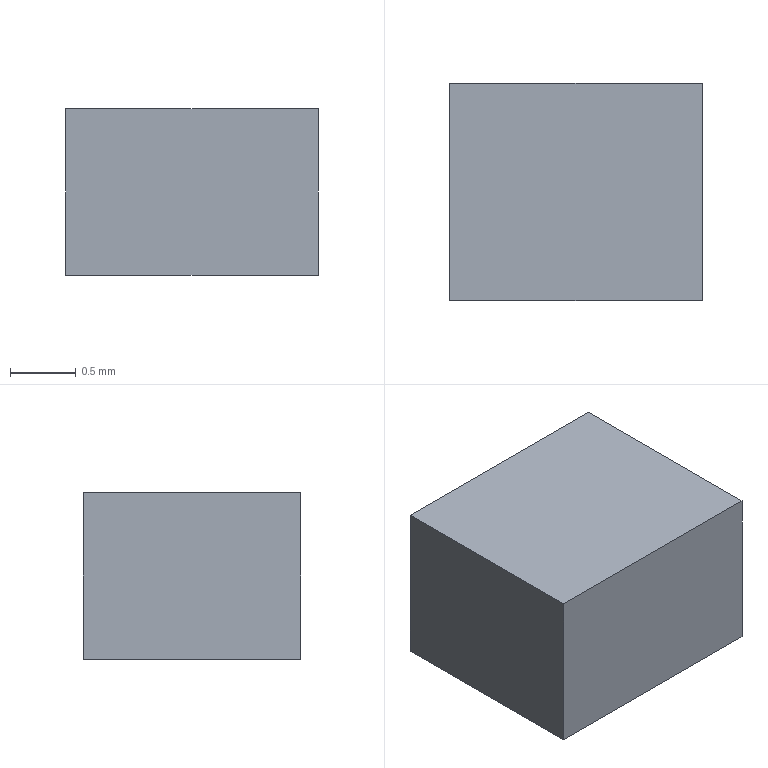Part | Creo | 1 solid | 6 faces | box 1.925 x 1.657 x 1.27 mm | volume 4.052 mm3 | plane 6
STEP:
#1=CARTESIAN_POINT('',(0.,0.,0.));
#2=DIRECTION('',(0.,0.,1.));
#3=DIRECTION('',(1.,0.,0.));
#4=AXIS2_PLACEMENT_3D('',#1,#2,#3);
#5=CARTESIAN_POINT('',(-0.9627,-0.8444,0.));
#6=VERTEX_POINT('',#5);
#7=CARTESIAN_POINT('',(0.9627,-0.8444,0.));
#8=VERTEX_POINT('',#7);
#9=CARTESIAN_POINT('',(-0.9627,-0.8444,0.));
#10=DIRECTION('',(1.,0.,0.));
#11=VECTOR('',#10,1.925);
#12=LINE('',#9,#11);
#13=EDGE_CURVE('',#6,#8,#12,.T.);
#14=ORIENTED_EDGE('',*,*,#13,.T.);
#15=CARTESIAN_POINT('',(0.9627,0.8127,0.));
#16=VERTEX_POINT('',#15);
#17=CARTESIAN_POINT('',(0.9627,-0.8444,0.));
#18=DIRECTION('',(0.,1.,0.));
#19=VECTOR('',#18,1.657);
#20=LINE('',#17,#19);
#21=EDGE_CURVE('',#8,#16,#20,.T.);
#22=ORIENTED_EDGE('',*,*,#21,.T.);
#23=CARTESIAN_POINT('',(-0.9627,0.8127,0.));
#24=VERTEX_POINT('',#23);
#25=CARTESIAN_POINT('',(0.9627,0.8127,0.));
#26=DIRECTION('',(-1.,0.,0.));
#27=VECTOR('',#26,1.925);
#28=LINE('',#25,#27);
#29=EDGE_CURVE('',#16,#24,#28,.T.);
#30=ORIENTED_EDGE('',*,*,#29,.T.);
#31=CARTESIAN_POINT('',(-0.9627,0.8127,0.));
#32=DIRECTION('',(0.,-1.,0.));
#33=VECTOR('',#32,1.657);
#34=LINE('',#31,#33);
#35=EDGE_CURVE('',#24,#6,#34,.T.);
#36=ORIENTED_EDGE('',*,*,#35,.T.);
#37=EDGE_LOOP('',(#14,#22,#30,#36));
#38=FACE_OUTER_BOUND('',#37,.F.);
#39=CARTESIAN_POINT('',(0.,0.,0.));
#40=DIRECTION('',(0.,0.,1.));
#41=DIRECTION('',(1.,0.,0.));
#42=AXIS2_PLACEMENT_3D('',#39,#40,#41);
#43=PLANE('',#42);
#44=ADVANCED_FACE('',(#38),#43,.F.);
#45=ORIENTED_EDGE('',*,*,#13,.F.);
#46=CARTESIAN_POINT('',(-0.9627,-0.8444,1.27));
#47=VERTEX_POINT('',#46);
#48=CARTESIAN_POINT('',(-0.9627,-0.8444,0.));
#49=DIRECTION('',(0.,0.,1.));
#50=VECTOR('',#49,1.27);
#51=LINE('',#48,#50);
#52=EDGE_CURVE('',#6,#47,#51,.T.);
#53=ORIENTED_EDGE('',*,*,#52,.T.);
#54=CARTESIAN_POINT('',(0.9627,-0.8444,1.27));
#55=VERTEX_POINT('',#54);
#56=CARTESIAN_POINT('',(-0.9627,-0.8444,1.27));
#57=DIRECTION('',(1.,0.,0.));
#58=VECTOR('',#57,1.925);
#59=LINE('',#56,#58);
#60=EDGE_CURVE('',#47,#55,#59,.T.);
#61=ORIENTED_EDGE('',*,*,#60,.T.);
#62=CARTESIAN_POINT('',(0.9627,-0.8444,0.));
#63=DIRECTION('',(0.,0.,1.));
#64=VECTOR('',#63,1.27);
#65=LINE('',#62,#64);
#66=EDGE_CURVE('',#8,#55,#65,.T.);
#67=ORIENTED_EDGE('',*,*,#66,.F.);
#68=EDGE_LOOP('',(#45,#53,#61,#67));
#69=FACE_OUTER_BOUND('',#68,.F.);
#70=CARTESIAN_POINT('',(-0.9627,-0.8444,0.));
#71=DIRECTION('',(0.,-1.,0.));
#72=DIRECTION('',(1.,0.,0.));
#73=AXIS2_PLACEMENT_3D('',#70,#71,#72);
#74=PLANE('',#73);
#75=ADVANCED_FACE('',(#69),#74,.T.);
#76=ORIENTED_EDGE('',*,*,#35,.F.);
#77=CARTESIAN_POINT('',(-0.9627,0.8127,1.27));
#78=VERTEX_POINT('',#77);
#79=CARTESIAN_POINT('',(-0.9627,0.8127,0.));
#80=DIRECTION('',(0.,0.,1.));
#81=VECTOR('',#80,1.27);
#82=LINE('',#79,#81);
#83=EDGE_CURVE('',#24,#78,#82,.T.);
#84=ORIENTED_EDGE('',*,*,#83,.T.);
#85=CARTESIAN_POINT('',(-0.9627,0.8127,1.27));
#86=DIRECTION('',(0.,-1.,0.));
#87=VECTOR('',#86,1.657);
#88=LINE('',#85,#87);
#89=EDGE_CURVE('',#78,#47,#88,.T.);
#90=ORIENTED_EDGE('',*,*,#89,.T.);
#91=ORIENTED_EDGE('',*,*,#52,.F.);
#92=EDGE_LOOP('',(#76,#84,#90,#91));
#93=FACE_OUTER_BOUND('',#92,.F.);
#94=CARTESIAN_POINT('',(-0.9627,0.8127,0.));
#95=DIRECTION('',(-1.,0.,0.));
#96=DIRECTION('',(0.,-1.,0.));
#97=AXIS2_PLACEMENT_3D('',#94,#95,#96);
#98=PLANE('',#97);
#99=ADVANCED_FACE('',(#93),#98,.T.);
#100=ORIENTED_EDGE('',*,*,#29,.F.);
#101=CARTESIAN_POINT('',(0.9627,0.8127,1.27));
#102=VERTEX_POINT('',#101);
#103=CARTESIAN_POINT('',(0.9627,0.8127,0.));
#104=DIRECTION('',(0.,0.,1.));
#105=VECTOR('',#104,1.27);
#106=LINE('',#103,#105);
#107=EDGE_CURVE('',#16,#102,#106,.T.);
#108=ORIENTED_EDGE('',*,*,#107,.T.);
#109=CARTESIAN_POINT('',(0.9627,0.8127,1.27));
#110=DIRECTION('',(-1.,0.,0.));
#111=VECTOR('',#110,1.925);
#112=LINE('',#109,#111);
#113=EDGE_CURVE('',#102,#78,#112,.T.);
#114=ORIENTED_EDGE('',*,*,#113,.T.);
#115=ORIENTED_EDGE('',*,*,#83,.F.);
#116=EDGE_LOOP('',(#100,#108,#114,#115));
#117=FACE_OUTER_BOUND('',#116,.F.);
#118=CARTESIAN_POINT('',(0.9627,0.8127,0.));
#119=DIRECTION('',(0.,1.,0.));
#120=DIRECTION('',(-1.,0.,0.));
#121=AXIS2_PLACEMENT_3D('',#118,#119,#120);
#122=PLANE('',#121);
#123=ADVANCED_FACE('',(#117),#122,.T.);
#124=ORIENTED_EDGE('',*,*,#21,.F.);
#125=ORIENTED_EDGE('',*,*,#66,.T.);
#126=CARTESIAN_POINT('',(0.9627,-0.8444,1.27));
#127=DIRECTION('',(0.,1.,0.));
#128=VECTOR('',#127,1.657);
#129=LINE('',#126,#128);
#130=EDGE_CURVE('',#55,#102,#129,.T.);
#131=ORIENTED_EDGE('',*,*,#130,.T.);
#132=ORIENTED_EDGE('',*,*,#107,.F.);
#133=EDGE_LOOP('',(#124,#125,#131,#132));
#134=FACE_OUTER_BOUND('',#133,.F.);
#135=CARTESIAN_POINT('',(0.9627,-0.8444,0.));
#136=DIRECTION('',(1.,0.,0.));
#137=DIRECTION('',(0.,1.,0.));
#138=AXIS2_PLACEMENT_3D('',#135,#136,#137);
#139=PLANE('',#138);
#140=ADVANCED_FACE('',(#134),#139,.T.);
#141=ORIENTED_EDGE('',*,*,#60,.F.);
#142=ORIENTED_EDGE('',*,*,#89,.F.);
#143=ORIENTED_EDGE('',*,*,#113,.F.);
#144=ORIENTED_EDGE('',*,*,#130,.F.);
#145=EDGE_LOOP('',(#141,#142,#143,#144));
#146=FACE_OUTER_BOUND('',#145,.F.);
#147=CARTESIAN_POINT('',(0.,0.,1.27));
#148=DIRECTION('',(0.,0.,1.));
#149=DIRECTION('',(1.,0.,0.));
#150=AXIS2_PLACEMENT_3D('',#147,#148,#149);
#151=PLANE('',#150);
#152=ADVANCED_FACE('',(#146),#151,.T.);
#153=CLOSED_SHELL('',(#44,#75,#99,#123,#140,#152));
#154=MANIFOLD_SOLID_BREP('',#153);
#155=(LENGTH_UNIT()NAMED_UNIT(*)SI_UNIT(.MILLI.,.METRE.));
#156=UNCERTAINTY_MEASURE_WITH_UNIT(LENGTH_MEASURE(0.000284),#155,'','');
#157=(NAMED_UNIT(*)PLANE_ANGLE_UNIT()SI_UNIT($,.RADIAN.));
#158=PLANE_ANGLE_MEASURE_WITH_UNIT(PLANE_ANGLE_MEASURE(0.01745),#157);
#159=(CONVERSION_BASED_UNIT('DEGREE',#158)NAMED_UNIT(*)PLANE_ANGLE_UNIT());
#160=(NAMED_UNIT(*)SI_UNIT($,.STERADIAN.)SOLID_ANGLE_UNIT());
#161=(GEOMETRIC_REPRESENTATION_CONTEXT(3)GLOBAL_UNCERTAINTY_ASSIGNED_CONTEXT((#156))GLOBAL_UNIT_ASSIGNED_CONTEXT((#155,#159,#160))REPRESENTATION_CONTEXT('',''));
#162=ADVANCED_BREP_SHAPE_REPRESENTATION('',(#4,#154),#161);